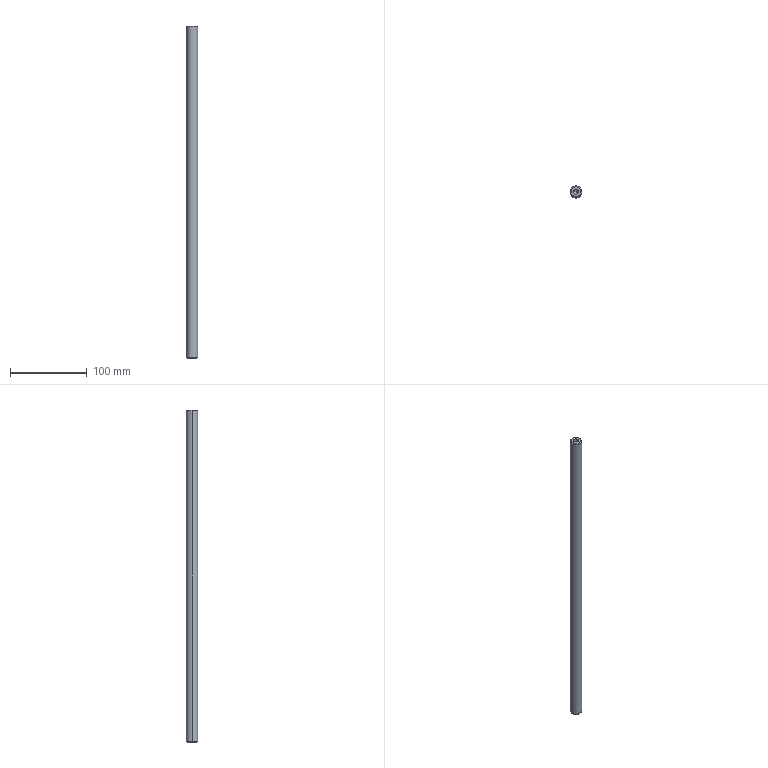Part | SolidWorks | features BaseBody 1 | 1 solid | 16 faces | box 15 x 15 x 432 mm | volume 74812 mm3 | cone 8 | cylinder 6 | plane 2 | commonest cylinder face diameters 6.8 x4 15 x2
STEP:
#1=CARTESIAN_POINT('',(3.4,0.,-196.25));
#2=VERTEX_POINT('',#1);
#3=CARTESIAN_POINT('',(-3.4,0.,-196.25));
#4=VERTEX_POINT('',#3);
#5=CARTESIAN_POINT('',(0.,0.,-196.25));
#6=DIRECTION('',(0.,0.,-1.));
#7=DIRECTION('',(-1.,0.,0.));
#8=AXIS2_PLACEMENT_3D('',#5,#6,#7);
#9=CIRCLE('',#8,3.4);
#10=EDGE_CURVE('',#2,#4,#9,.T.);
#11=ORIENTED_EDGE('',*,*,#10,.F.);
#12=CARTESIAN_POINT('',(3.4,0.,-216.));
#13=VERTEX_POINT('',#12);
#14=CARTESIAN_POINT('',(3.4,0.,-216.));
#15=DIRECTION('',(0.,0.,-1.));
#16=VECTOR('',#15,1000.);
#17=LINE('',#14,#16);
#18=EDGE_CURVE('',#2,#13,#17,.T.);
#19=ORIENTED_EDGE('',*,*,#18,.T.);
#20=CARTESIAN_POINT('',(-3.4,0.,-216.));
#21=VERTEX_POINT('',#20);
#22=CARTESIAN_POINT('',(0.,0.,-216.));
#23=DIRECTION('',(0.,0.,-1.));
#24=DIRECTION('',(-1.,0.,0.));
#25=AXIS2_PLACEMENT_3D('',#22,#23,#24);
#26=CIRCLE('',#25,3.4);
#27=EDGE_CURVE('',#13,#21,#26,.T.);
#28=ORIENTED_EDGE('',*,*,#27,.T.);
#29=CARTESIAN_POINT('',(-3.4,0.,-216.));
#30=DIRECTION('',(0.,0.,-1.));
#31=VECTOR('',#30,1000.);
#32=LINE('',#29,#31);
#33=EDGE_CURVE('',#4,#21,#32,.T.);
#34=ORIENTED_EDGE('',*,*,#33,.F.);
#35=EDGE_LOOP('',(#11,#19,#28,#34));
#36=FACE_OUTER_BOUND('',#35,.T.);
#37=CARTESIAN_POINT('',(0.,0.,-216.));
#38=DIRECTION('',(0.,0.,-1.));
#39=DIRECTION('',(-1.,0.,0.));
#40=AXIS2_PLACEMENT_3D('',#37,#38,#39);
#41=CYLINDRICAL_SURFACE('',#40,3.4);
#42=ADVANCED_FACE('',(#36),#41,.F.);
#43=CARTESIAN_POINT('',(0.,0.,-194.207));
#44=VERTEX_POINT('',#43);
#45=CARTESIAN_POINT('',(-3.4,0.,-196.25));
#46=DIRECTION('',(-0.8572,0.,-0.515));
#47=VECTOR('',#46,1000.);
#48=LINE('',#45,#47);
#49=EDGE_CURVE('',#44,#4,#48,.T.);
#50=ORIENTED_EDGE('',*,*,#49,.F.);
#51=CARTESIAN_POINT('',(3.4,0.,-196.25));
#52=DIRECTION('',(0.8572,0.,-0.515));
#53=VECTOR('',#52,1000.);
#54=LINE('',#51,#53);
#55=EDGE_CURVE('',#44,#2,#54,.T.);
#56=ORIENTED_EDGE('',*,*,#55,.T.);
#57=ORIENTED_EDGE('',*,*,#10,.T.);
#58=EDGE_LOOP('',(#50,#56,#57));
#59=FACE_OUTER_BOUND('',#58,.T.);
#60=CARTESIAN_POINT('',(0.,0.,-196.25));
#61=DIRECTION('',(0.,0.,-1.));
#62=DIRECTION('',(-1.,0.,0.));
#63=AXIS2_PLACEMENT_3D('',#60,#61,#62);
#64=CONICAL_SURFACE('',#63,3.4,1.03);
#65=ADVANCED_FACE('',(#59),#64,.F.);
#66=CARTESIAN_POINT('',(-3.4,0.,196.25));
#67=VERTEX_POINT('',#66);
#68=CARTESIAN_POINT('',(3.4,0.,196.25));
#69=VERTEX_POINT('',#68);
#70=CARTESIAN_POINT('',(0.,0.,196.25));
#71=DIRECTION('',(0.,0.,1.));
#72=DIRECTION('',(1.,0.,0.));
#73=AXIS2_PLACEMENT_3D('',#70,#71,#72);
#74=CIRCLE('',#73,3.4);
#75=EDGE_CURVE('',#67,#69,#74,.T.);
#76=ORIENTED_EDGE('',*,*,#75,.F.);
#77=CARTESIAN_POINT('',(-3.4,0.,216.));
#78=VERTEX_POINT('',#77);
#79=CARTESIAN_POINT('',(-3.4,0.,216.));
#80=DIRECTION('',(0.,0.,1.));
#81=VECTOR('',#80,1000.);
#82=LINE('',#79,#81);
#83=EDGE_CURVE('',#67,#78,#82,.T.);
#84=ORIENTED_EDGE('',*,*,#83,.T.);
#85=CARTESIAN_POINT('',(3.4,0.,216.));
#86=VERTEX_POINT('',#85);
#87=CARTESIAN_POINT('',(0.,0.,216.));
#88=DIRECTION('',(0.,0.,1.));
#89=DIRECTION('',(1.,0.,0.));
#90=AXIS2_PLACEMENT_3D('',#87,#88,#89);
#91=CIRCLE('',#90,3.4);
#92=EDGE_CURVE('',#78,#86,#91,.T.);
#93=ORIENTED_EDGE('',*,*,#92,.T.);
#94=CARTESIAN_POINT('',(3.4,0.,216.));
#95=DIRECTION('',(0.,0.,1.));
#96=VECTOR('',#95,1000.);
#97=LINE('',#94,#96);
#98=EDGE_CURVE('',#69,#86,#97,.T.);
#99=ORIENTED_EDGE('',*,*,#98,.F.);
#100=EDGE_LOOP('',(#76,#84,#93,#99));
#101=FACE_OUTER_BOUND('',#100,.T.);
#102=CARTESIAN_POINT('',(0.,0.,216.));
#103=DIRECTION('',(0.,0.,1.));
#104=DIRECTION('',(1.,0.,0.));
#105=AXIS2_PLACEMENT_3D('',#102,#103,#104);
#106=CYLINDRICAL_SURFACE('',#105,3.4);
#107=ADVANCED_FACE('',(#101),#106,.F.);
#108=CARTESIAN_POINT('',(0.,0.,194.207));
#109=VERTEX_POINT('',#108);
#110=CARTESIAN_POINT('',(3.4,0.,196.25));
#111=DIRECTION('',(0.8572,0.,0.515));
#112=VECTOR('',#111,1000.);
#113=LINE('',#110,#112);
#114=EDGE_CURVE('',#109,#69,#113,.T.);
#115=ORIENTED_EDGE('',*,*,#114,.F.);
#116=CARTESIAN_POINT('',(-3.4,0.,196.25));
#117=DIRECTION('',(-0.8572,0.,0.515));
#118=VECTOR('',#117,1000.);
#119=LINE('',#116,#118);
#120=EDGE_CURVE('',#109,#67,#119,.T.);
#121=ORIENTED_EDGE('',*,*,#120,.T.);
#122=ORIENTED_EDGE('',*,*,#75,.T.);
#123=EDGE_LOOP('',(#115,#121,#122));
#124=FACE_OUTER_BOUND('',#123,.T.);
#125=CARTESIAN_POINT('',(0.,0.,196.25));
#126=DIRECTION('',(0.,0.,1.));
#127=DIRECTION('',(1.,0.,0.));
#128=AXIS2_PLACEMENT_3D('',#125,#126,#127);
#129=CONICAL_SURFACE('',#128,3.4,1.03);
#130=ADVANCED_FACE('',(#124),#129,.F.);
#131=CARTESIAN_POINT('',(6.5,0.,216.));
#132=VERTEX_POINT('',#131);
#133=CARTESIAN_POINT('',(-6.5,0.,216.));
#134=VERTEX_POINT('',#133);
#135=CARTESIAN_POINT('',(0.,0.,216.));
#136=DIRECTION('',(0.,0.,1.));
#137=DIRECTION('',(1.,0.,0.));
#138=AXIS2_PLACEMENT_3D('',#135,#136,#137);
#139=CIRCLE('',#138,6.5);
#140=EDGE_CURVE('',#132,#134,#139,.T.);
#141=ORIENTED_EDGE('',*,*,#140,.F.);
#142=CARTESIAN_POINT('',(7.5,0.,215.));
#143=VERTEX_POINT('',#142);
#144=CARTESIAN_POINT('',(6.5,0.,216.));
#145=DIRECTION('',(0.7071,0.,-0.7071));
#146=VECTOR('',#145,1000.);
#147=LINE('',#144,#146);
#148=EDGE_CURVE('',#132,#143,#147,.T.);
#149=ORIENTED_EDGE('',*,*,#148,.T.);
#150=CARTESIAN_POINT('',(-7.5,0.,215.));
#151=VERTEX_POINT('',#150);
#152=CARTESIAN_POINT('',(0.,0.,215.));
#153=DIRECTION('',(0.,0.,-1.));
#154=DIRECTION('',(1.,0.,0.));
#155=AXIS2_PLACEMENT_3D('',#152,#153,#154);
#156=CIRCLE('',#155,7.5);
#157=EDGE_CURVE('',#151,#143,#156,.T.);
#158=ORIENTED_EDGE('',*,*,#157,.F.);
#159=CARTESIAN_POINT('',(-6.5,0.,216.));
#160=DIRECTION('',(-0.7071,0.,-0.7071));
#161=VECTOR('',#160,1000.);
#162=LINE('',#159,#161);
#163=EDGE_CURVE('',#134,#151,#162,.T.);
#164=ORIENTED_EDGE('',*,*,#163,.F.);
#165=EDGE_LOOP('',(#141,#149,#158,#164));
#166=FACE_OUTER_BOUND('',#165,.T.);
#167=CARTESIAN_POINT('',(0.,0.,216.));
#168=DIRECTION('',(0.,0.,-1.));
#169=DIRECTION('',(-1.,0.,0.));
#170=AXIS2_PLACEMENT_3D('',#167,#168,#169);
#171=CONICAL_SURFACE('',#170,6.5,0.7854);
#172=ADVANCED_FACE('',(#166),#171,.T.);
#173=CARTESIAN_POINT('',(-6.5,0.,-216.));
#174=VERTEX_POINT('',#173);
#175=CARTESIAN_POINT('',(6.5,0.,-216.));
#176=VERTEX_POINT('',#175);
#177=CARTESIAN_POINT('',(0.,0.,-216.));
#178=DIRECTION('',(0.,0.,-1.));
#179=DIRECTION('',(1.,0.,0.));
#180=AXIS2_PLACEMENT_3D('',#177,#178,#179);
#181=CIRCLE('',#180,6.5);
#182=EDGE_CURVE('',#174,#176,#181,.T.);
#183=ORIENTED_EDGE('',*,*,#182,.F.);
#184=CARTESIAN_POINT('',(-7.5,0.,-215.));
#185=VERTEX_POINT('',#184);
#186=CARTESIAN_POINT('',(-7.5,0.,-215.));
#187=DIRECTION('',(-0.7071,0.,0.7071));
#188=VECTOR('',#187,1000.);
#189=LINE('',#186,#188);
#190=EDGE_CURVE('',#174,#185,#189,.T.);
#191=ORIENTED_EDGE('',*,*,#190,.T.);
#192=CARTESIAN_POINT('',(7.5,0.,-215.));
#193=VERTEX_POINT('',#192);
#194=CARTESIAN_POINT('',(0.,0.,-215.));
#195=DIRECTION('',(0.,0.,1.));
#196=DIRECTION('',(1.,0.,0.));
#197=AXIS2_PLACEMENT_3D('',#194,#195,#196);
#198=CIRCLE('',#197,7.5);
#199=EDGE_CURVE('',#193,#185,#198,.T.);
#200=ORIENTED_EDGE('',*,*,#199,.F.);
#201=CARTESIAN_POINT('',(7.5,0.,-215.));
#202=DIRECTION('',(0.7071,0.,0.7071));
#203=VECTOR('',#202,1000.);
#204=LINE('',#201,#203);
#205=EDGE_CURVE('',#176,#193,#204,.T.);
#206=ORIENTED_EDGE('',*,*,#205,.F.);
#207=EDGE_LOOP('',(#183,#191,#200,#206));
#208=FACE_OUTER_BOUND('',#207,.T.);
#209=CARTESIAN_POINT('',(0.,0.,-215.));
#210=DIRECTION('',(0.,0.,1.));
#211=DIRECTION('',(1.,0.,0.));
#212=AXIS2_PLACEMENT_3D('',#209,#210,#211);
#213=CONICAL_SURFACE('',#212,7.5,0.7854);
#214=ADVANCED_FACE('',(#208),#213,.T.);
#215=ORIENTED_EDGE('',*,*,#157,.T.);
#216=CARTESIAN_POINT('',(7.5,0.,216.));
#217=DIRECTION('',(0.,0.,-1.));
#218=VECTOR('',#217,1000.);
#219=LINE('',#216,#218);
#220=EDGE_CURVE('',#143,#193,#219,.T.);
#221=ORIENTED_EDGE('',*,*,#220,.T.);
#222=ORIENTED_EDGE('',*,*,#199,.T.);
#223=CARTESIAN_POINT('',(-7.5,0.,216.));
#224=DIRECTION('',(0.,0.,-1.));
#225=VECTOR('',#224,1000.);
#226=LINE('',#223,#225);
#227=EDGE_CURVE('',#151,#185,#226,.T.);
#228=ORIENTED_EDGE('',*,*,#227,.F.);
#229=EDGE_LOOP('',(#215,#221,#222,#228));
#230=FACE_OUTER_BOUND('',#229,.T.);
#231=CARTESIAN_POINT('',(0.,0.,216.));
#232=DIRECTION('',(0.,0.,-1.));
#233=DIRECTION('',(-1.,0.,0.));
#234=AXIS2_PLACEMENT_3D('',#231,#232,#233);
#235=CYLINDRICAL_SURFACE('',#234,7.5);
#236=ADVANCED_FACE('',(#230),#235,.T.);
#237=ORIENTED_EDGE('',*,*,#220,.F.);
#238=CARTESIAN_POINT('',(0.,0.,215.));
#239=DIRECTION('',(0.,0.,-1.));
#240=DIRECTION('',(1.,0.,0.));
#241=AXIS2_PLACEMENT_3D('',#238,#239,#240);
#242=CIRCLE('',#241,7.5);
#243=EDGE_CURVE('',#143,#151,#242,.T.);
#244=ORIENTED_EDGE('',*,*,#243,.T.);
#245=ORIENTED_EDGE('',*,*,#227,.T.);
#246=CARTESIAN_POINT('',(0.,0.,-215.));
#247=DIRECTION('',(0.,0.,1.));
#248=DIRECTION('',(1.,0.,0.));
#249=AXIS2_PLACEMENT_3D('',#246,#247,#248);
#250=CIRCLE('',#249,7.5);
#251=EDGE_CURVE('',#185,#193,#250,.T.);
#252=ORIENTED_EDGE('',*,*,#251,.T.);
#253=EDGE_LOOP('',(#237,#244,#245,#252));
#254=FACE_OUTER_BOUND('',#253,.T.);
#255=CARTESIAN_POINT('',(0.,0.,216.));
#256=DIRECTION('',(0.,0.,-1.));
#257=DIRECTION('',(-1.,0.,0.));
#258=AXIS2_PLACEMENT_3D('',#255,#256,#257);
#259=CYLINDRICAL_SURFACE('',#258,7.5);
#260=ADVANCED_FACE('',(#254),#259,.T.);
#261=CARTESIAN_POINT('',(0.,0.,216.));
#262=DIRECTION('',(0.,0.,1.));
#263=DIRECTION('',(1.,0.,0.));
#264=AXIS2_PLACEMENT_3D('',#261,#262,#263);
#265=CIRCLE('',#264,3.4);
#266=EDGE_CURVE('',#86,#78,#265,.T.);
#267=ORIENTED_EDGE('',*,*,#266,.F.);
#268=ORIENTED_EDGE('',*,*,#92,.F.);
#269=EDGE_LOOP('',(#267,#268));
#270=FACE_BOUND('',#269,.T.);
#271=CARTESIAN_POINT('',(0.,0.,216.));
#272=DIRECTION('',(0.,0.,1.));
#273=DIRECTION('',(1.,0.,0.));
#274=AXIS2_PLACEMENT_3D('',#271,#272,#273);
#275=CIRCLE('',#274,6.5);
#276=EDGE_CURVE('',#134,#132,#275,.T.);
#277=ORIENTED_EDGE('',*,*,#276,.T.);
#278=ORIENTED_EDGE('',*,*,#140,.T.);
#279=EDGE_LOOP('',(#277,#278));
#280=FACE_OUTER_BOUND('',#279,.T.);
#281=CARTESIAN_POINT('',(0.,0.,216.));
#282=DIRECTION('',(0.,0.,1.));
#283=DIRECTION('',(1.,0.,0.));
#284=AXIS2_PLACEMENT_3D('',#281,#282,#283);
#285=PLANE('',#284);
#286=ADVANCED_FACE('',(#270,#280),#285,.T.);
#287=CARTESIAN_POINT('',(0.,0.,-216.));
#288=DIRECTION('',(0.,0.,-1.));
#289=DIRECTION('',(-1.,0.,0.));
#290=AXIS2_PLACEMENT_3D('',#287,#288,#289);
#291=CIRCLE('',#290,3.4);
#292=EDGE_CURVE('',#21,#13,#291,.T.);
#293=ORIENTED_EDGE('',*,*,#292,.F.);
#294=ORIENTED_EDGE('',*,*,#27,.F.);
#295=EDGE_LOOP('',(#293,#294));
#296=FACE_BOUND('',#295,.T.);
#297=CARTESIAN_POINT('',(0.,0.,-216.));
#298=DIRECTION('',(0.,0.,-1.));
#299=DIRECTION('',(1.,0.,0.));
#300=AXIS2_PLACEMENT_3D('',#297,#298,#299);
#301=CIRCLE('',#300,6.5);
#302=EDGE_CURVE('',#176,#174,#301,.T.);
#303=ORIENTED_EDGE('',*,*,#302,.T.);
#304=ORIENTED_EDGE('',*,*,#182,.T.);
#305=EDGE_LOOP('',(#303,#304));
#306=FACE_OUTER_BOUND('',#305,.T.);
#307=CARTESIAN_POINT('',(0.,0.,-216.));
#308=DIRECTION('',(0.,0.,1.));
#309=DIRECTION('',(1.,0.,0.));
#310=AXIS2_PLACEMENT_3D('',#307,#308,#309);
#311=PLANE('',#310);
#312=ADVANCED_FACE('',(#296,#306),#311,.F.);
#313=ORIENTED_EDGE('',*,*,#190,.F.);
#314=ORIENTED_EDGE('',*,*,#302,.F.);
#315=ORIENTED_EDGE('',*,*,#205,.T.);
#316=ORIENTED_EDGE('',*,*,#251,.F.);
#317=EDGE_LOOP('',(#313,#314,#315,#316));
#318=FACE_OUTER_BOUND('',#317,.T.);
#319=CARTESIAN_POINT('',(0.,0.,-215.));
#320=DIRECTION('',(0.,0.,1.));
#321=DIRECTION('',(1.,0.,0.));
#322=AXIS2_PLACEMENT_3D('',#319,#320,#321);
#323=CONICAL_SURFACE('',#322,7.5,0.7854);
#324=ADVANCED_FACE('',(#318),#323,.T.);
#325=ORIENTED_EDGE('',*,*,#148,.F.);
#326=ORIENTED_EDGE('',*,*,#276,.F.);
#327=ORIENTED_EDGE('',*,*,#163,.T.);
#328=ORIENTED_EDGE('',*,*,#243,.F.);
#329=EDGE_LOOP('',(#325,#326,#327,#328));
#330=FACE_OUTER_BOUND('',#329,.T.);
#331=CARTESIAN_POINT('',(0.,0.,216.));
#332=DIRECTION('',(0.,0.,-1.));
#333=DIRECTION('',(-1.,0.,0.));
#334=AXIS2_PLACEMENT_3D('',#331,#332,#333);
#335=CONICAL_SURFACE('',#334,6.5,0.7854);
#336=ADVANCED_FACE('',(#330),#335,.T.);
#337=ORIENTED_EDGE('',*,*,#120,.F.);
#338=ORIENTED_EDGE('',*,*,#114,.T.);
#339=CARTESIAN_POINT('',(0.,0.,196.25));
#340=DIRECTION('',(0.,0.,1.));
#341=DIRECTION('',(1.,0.,0.));
#342=AXIS2_PLACEMENT_3D('',#339,#340,#341);
#343=CIRCLE('',#342,3.4);
#344=EDGE_CURVE('',#69,#67,#343,.T.);
#345=ORIENTED_EDGE('',*,*,#344,.T.);
#346=EDGE_LOOP('',(#337,#338,#345));
#347=FACE_OUTER_BOUND('',#346,.T.);
#348=CARTESIAN_POINT('',(0.,0.,196.25));
#349=DIRECTION('',(0.,0.,1.));
#350=DIRECTION('',(1.,0.,0.));
#351=AXIS2_PLACEMENT_3D('',#348,#349,#350);
#352=CONICAL_SURFACE('',#351,3.4,1.03);
#353=ADVANCED_FACE('',(#347),#352,.F.);
#354=ORIENTED_EDGE('',*,*,#83,.F.);
#355=ORIENTED_EDGE('',*,*,#344,.F.);
#356=ORIENTED_EDGE('',*,*,#98,.T.);
#357=ORIENTED_EDGE('',*,*,#266,.T.);
#358=EDGE_LOOP('',(#354,#355,#356,#357));
#359=FACE_OUTER_BOUND('',#358,.T.);
#360=CARTESIAN_POINT('',(0.,0.,216.));
#361=DIRECTION('',(0.,0.,1.));
#362=DIRECTION('',(1.,0.,0.));
#363=AXIS2_PLACEMENT_3D('',#360,#361,#362);
#364=CYLINDRICAL_SURFACE('',#363,3.4);
#365=ADVANCED_FACE('',(#359),#364,.F.);
#366=ORIENTED_EDGE('',*,*,#55,.F.);
#367=ORIENTED_EDGE('',*,*,#49,.T.);
#368=CARTESIAN_POINT('',(0.,0.,-196.25));
#369=DIRECTION('',(0.,0.,-1.));
#370=DIRECTION('',(-1.,0.,0.));
#371=AXIS2_PLACEMENT_3D('',#368,#369,#370);
#372=CIRCLE('',#371,3.4);
#373=EDGE_CURVE('',#4,#2,#372,.T.);
#374=ORIENTED_EDGE('',*,*,#373,.T.);
#375=EDGE_LOOP('',(#366,#367,#374));
#376=FACE_OUTER_BOUND('',#375,.T.);
#377=CARTESIAN_POINT('',(0.,0.,-196.25));
#378=DIRECTION('',(0.,0.,-1.));
#379=DIRECTION('',(-1.,0.,0.));
#380=AXIS2_PLACEMENT_3D('',#377,#378,#379);
#381=CONICAL_SURFACE('',#380,3.4,1.03);
#382=ADVANCED_FACE('',(#376),#381,.F.);
#383=ORIENTED_EDGE('',*,*,#18,.F.);
#384=ORIENTED_EDGE('',*,*,#373,.F.);
#385=ORIENTED_EDGE('',*,*,#33,.T.);
#386=ORIENTED_EDGE('',*,*,#292,.T.);
#387=EDGE_LOOP('',(#383,#384,#385,#386));
#388=FACE_OUTER_BOUND('',#387,.T.);
#389=CARTESIAN_POINT('',(0.,0.,-216.));
#390=DIRECTION('',(0.,0.,-1.));
#391=DIRECTION('',(-1.,0.,0.));
#392=AXIS2_PLACEMENT_3D('',#389,#390,#391);
#393=CYLINDRICAL_SURFACE('',#392,3.4);
#394=ADVANCED_FACE('',(#388),#393,.F.);
#395=CLOSED_SHELL('',(#42,#65,#107,#130,#172,#214,#236,#260,#286,#312,#324,#336,#353,#365,#382,#394));
#396=MANIFOLD_SOLID_BREP('',#395);
#397=CARTESIAN_POINT('',(0.,0.,0.));
#398=DIRECTION('',(0.,0.,1.));
#399=DIRECTION('',(1.,0.,0.));
#400=AXIS2_PLACEMENT_3D('',#397,#398,#399);
#401=(LENGTH_UNIT()NAMED_UNIT(*)SI_UNIT(.MILLI.,.METRE.));
#402=UNCERTAINTY_MEASURE_WITH_UNIT(LENGTH_MEASURE(0.00001),#401,'','');
#403=(NAMED_UNIT(*)PLANE_ANGLE_UNIT()SI_UNIT($,.RADIAN.));
#404=(NAMED_UNIT(*)SI_UNIT($,.STERADIAN.)SOLID_ANGLE_UNIT());
#405=(GEOMETRIC_REPRESENTATION_CONTEXT(3)GLOBAL_UNCERTAINTY_ASSIGNED_CONTEXT((#402))GLOBAL_UNIT_ASSIGNED_CONTEXT((#401,#403,#404))REPRESENTATION_CONTEXT('',''));
#406=ADVANCED_BREP_SHAPE_REPRESENTATION('',(#396,#400),#405);